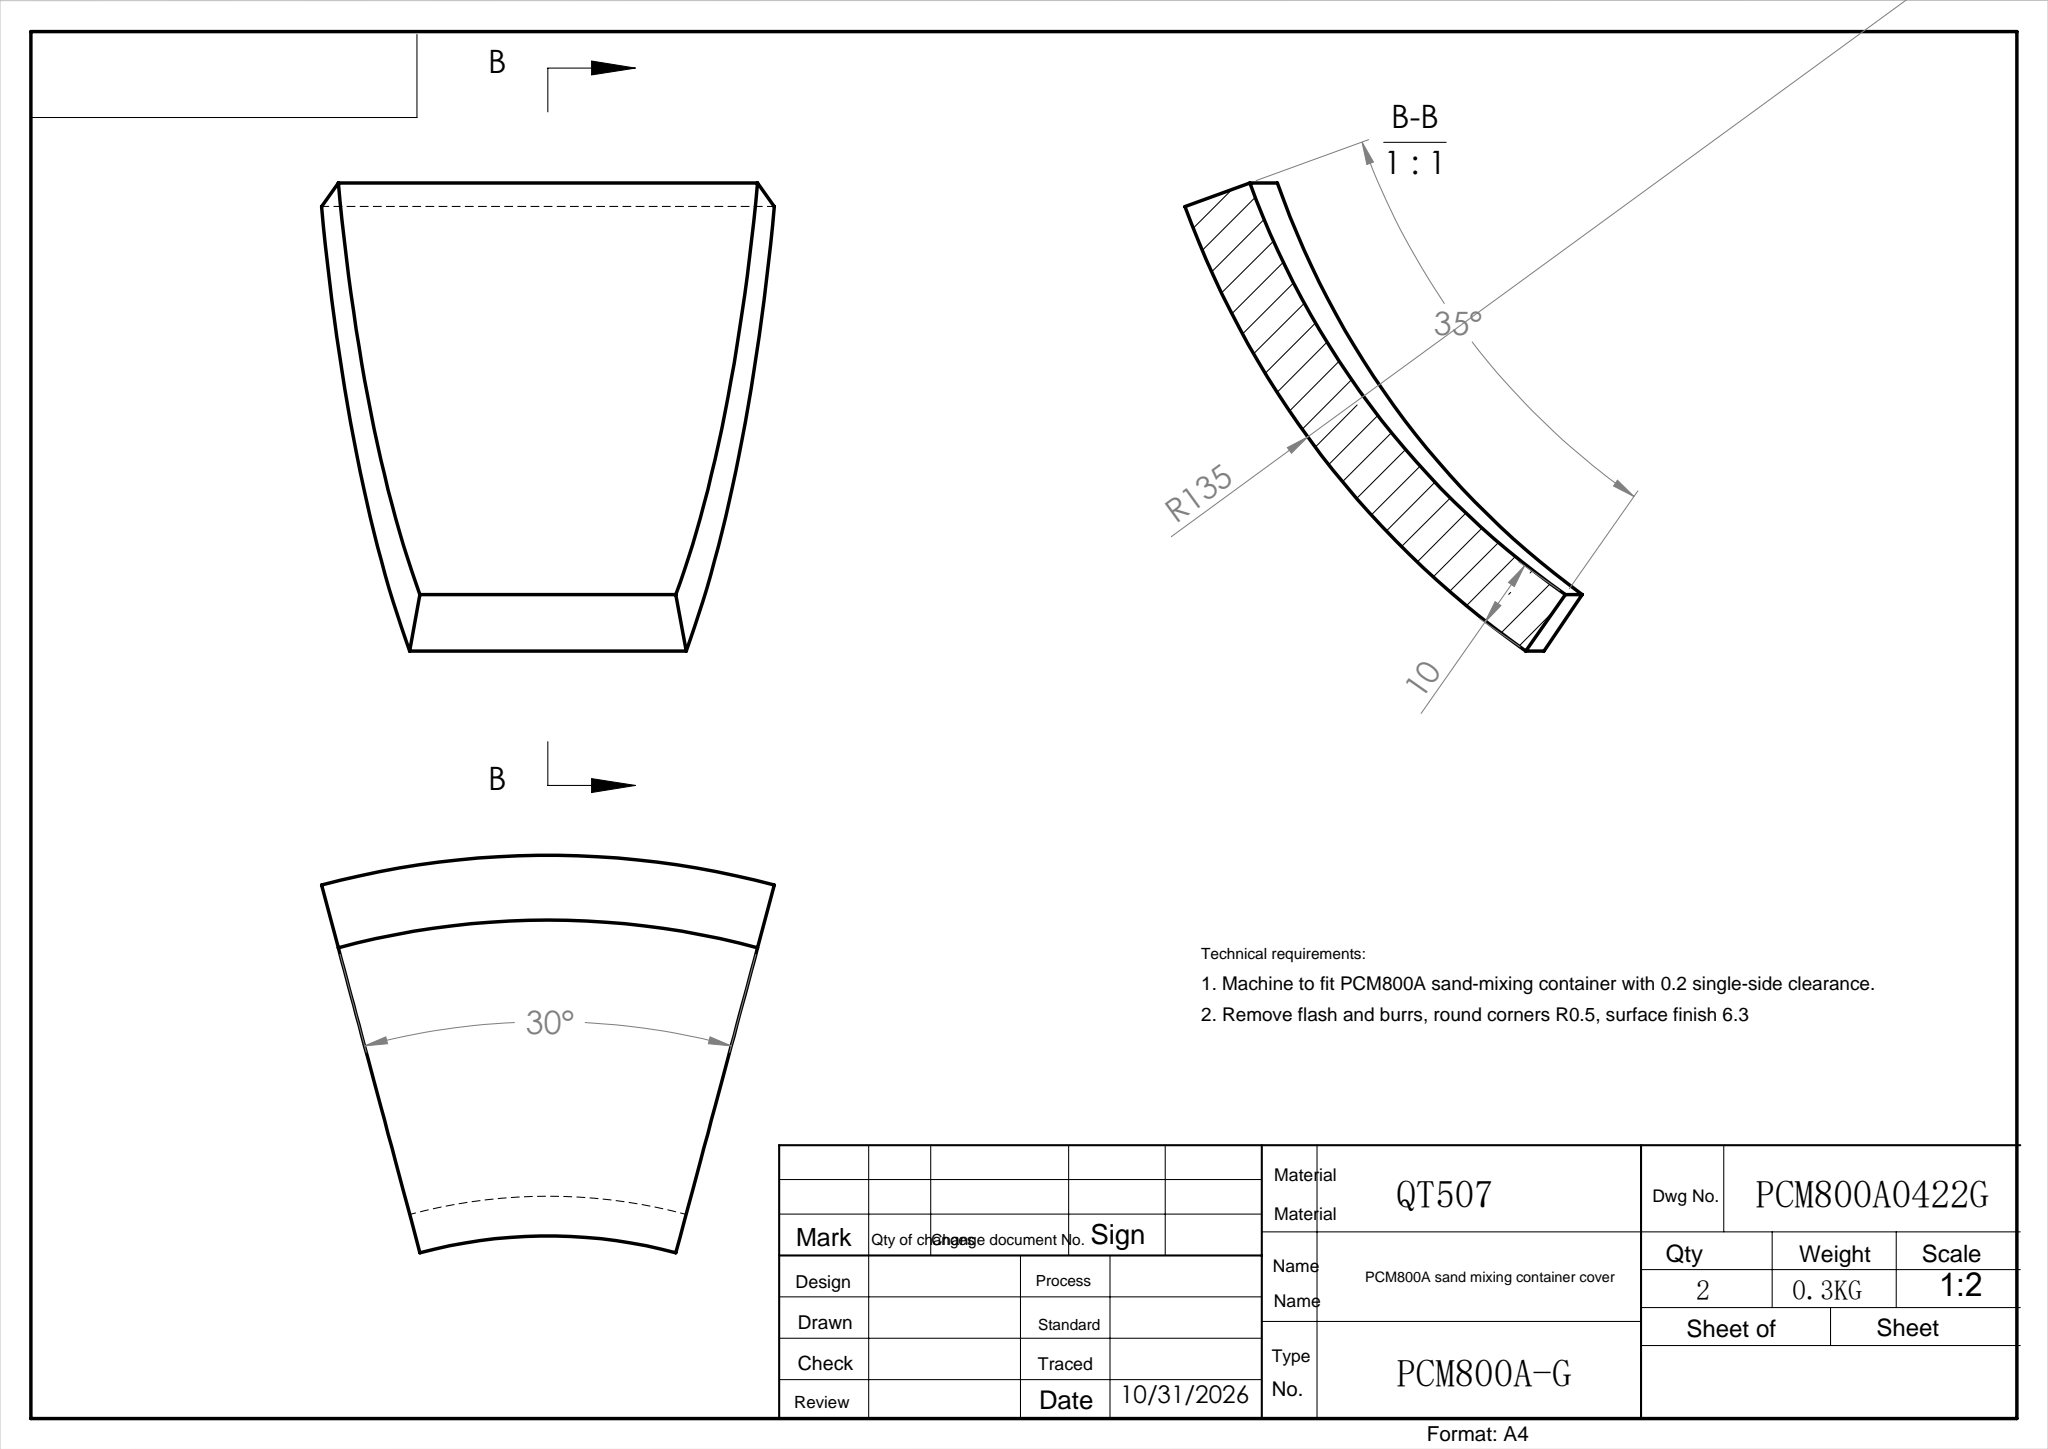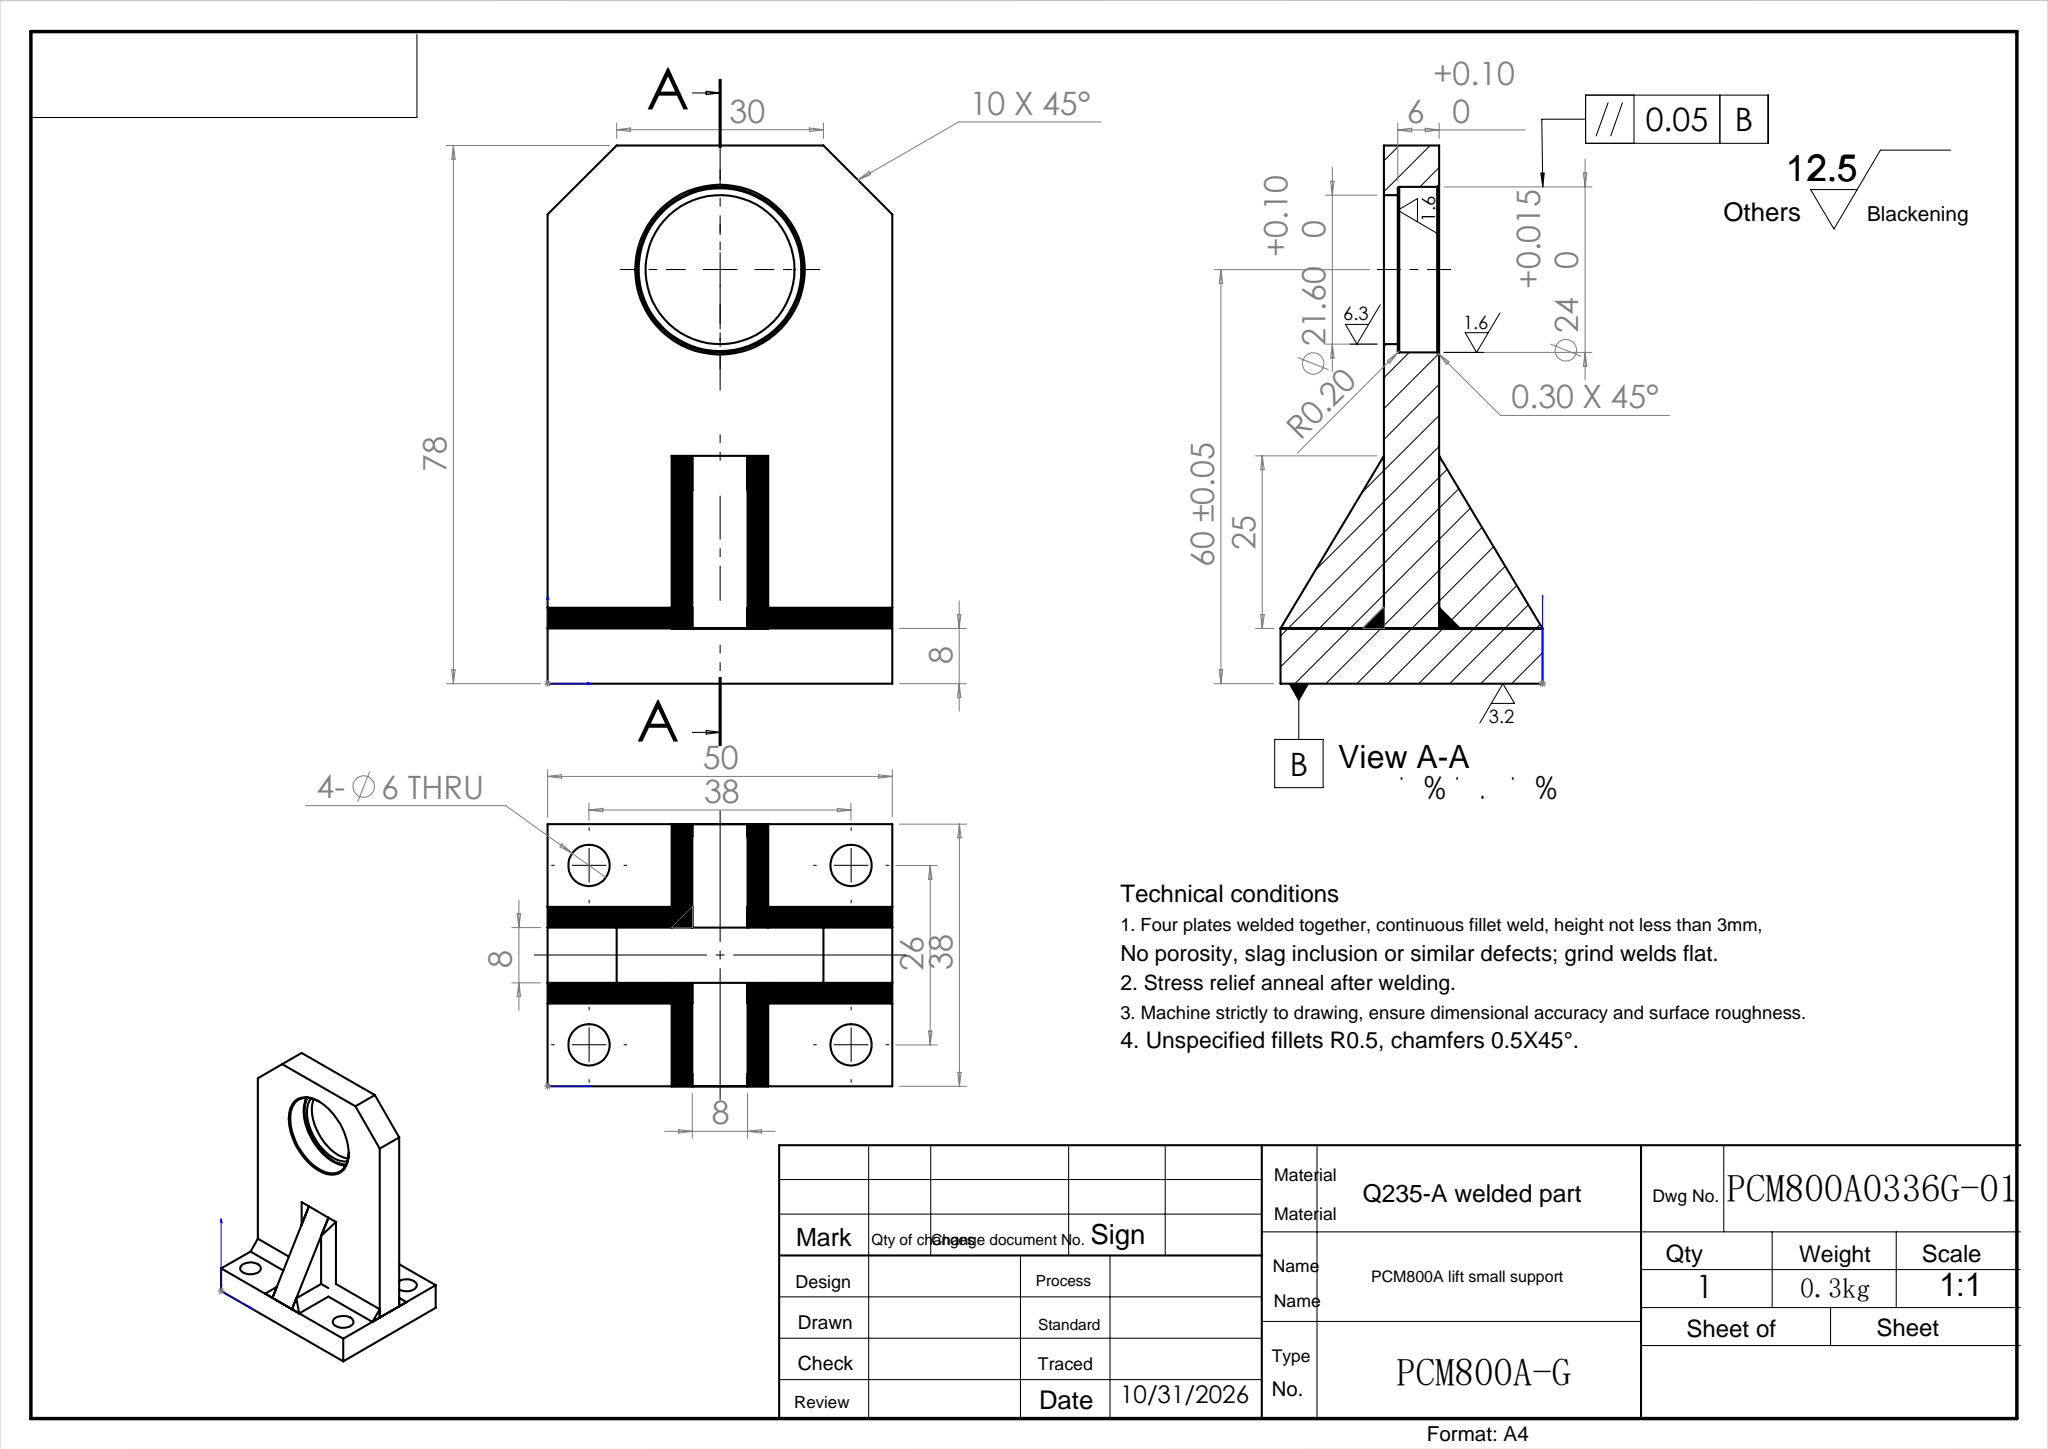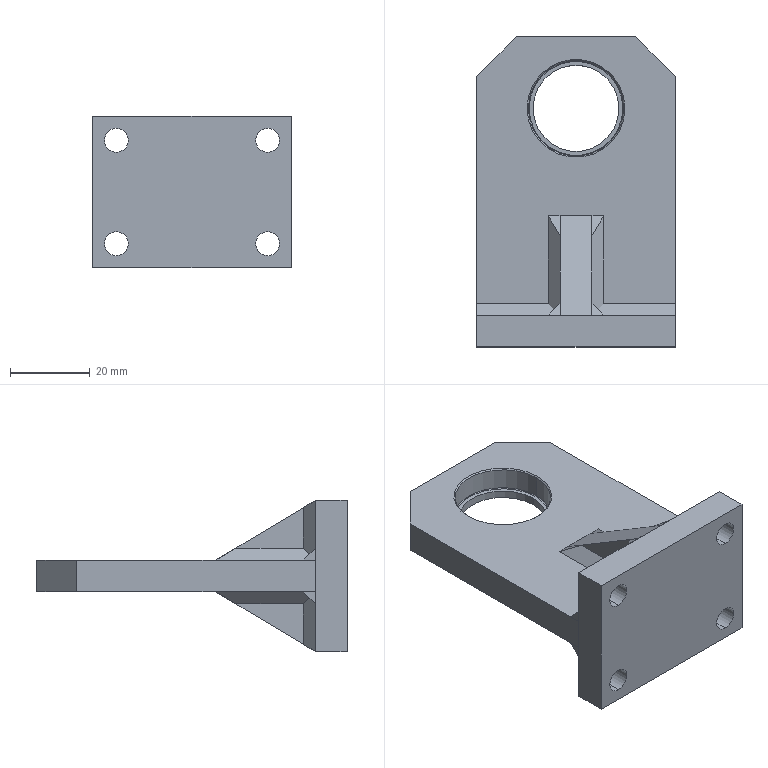Part | SolidWorks | features Cut 3, Chamfer 2, Gusset 2, WeldBeadFeat 2, Boss 1, Extrusion 1, Fillet 1, WeldmentFeature 1 | 10 solids | 79 faces | box 50 x 78 x 38 mm | volume 42138 mm3 | plane 63 | cylinder 12 | torus 2 | cone 2 | commonest cylinder face diameters 6 x8 21.6 x2 24 x2